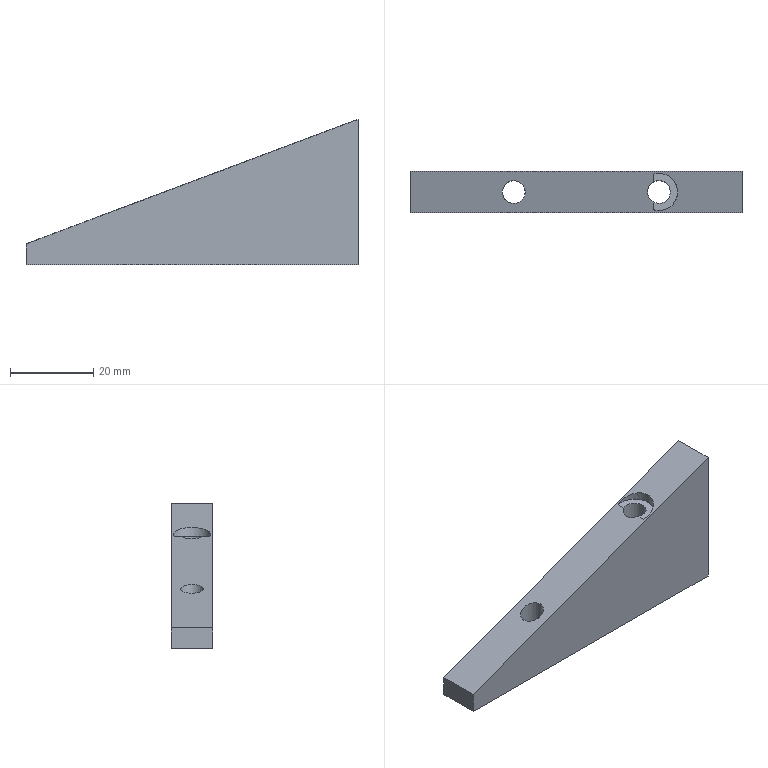Part | NX | 1 solid | 12 faces | box 80 x 10 x 35 mm | volume 14711 mm3 | plane 7 | cylinder 4 | cone 1 | commonest cylinder face diameters 5.5 x2 5 x1 9 x1
STEP:
#1=CARTESIAN_POINT('',(58.667,0.7021,27.));
#2=VERTEX_POINT('',#1);
#3=CARTESIAN_POINT('',(58.667,9.298,27.));
#4=VERTEX_POINT('',#3);
#5=CARTESIAN_POINT('',(60.,5.,27.));
#6=DIRECTION('',(0.,0.,1.));
#7=DIRECTION('',(1.,0.,0.));
#8=AXIS2_PLACEMENT_3D('',#5,#6,#7);
#9=CIRCLE('',#8,4.5);
#10=EDGE_CURVE('',#2,#4,#9,.T.);
#11=ORIENTED_EDGE('',*,*,#10,.F.);
#12=CARTESIAN_POINT('',(64.5,5.,29.188));
#13=VERTEX_POINT('',#12);
#14=CARTESIAN_POINT('',(58.667,0.7021,27.));
#15=CARTESIAN_POINT('',(61.832,-0.2799,28.187));
#16=CARTESIAN_POINT('',(64.5,1.686,29.188));
#17=CARTESIAN_POINT('',(64.5,5.,29.188));
#18=(BOUNDED_CURVE()B_SPLINE_CURVE(3,(#14,#15,#16,#17),.UNSPECIFIED.,.F.,.F.)B_SPLINE_CURVE_WITH_KNOTS((4,4),(0.,1.),.PIECEWISE_BEZIER_KNOTS.)CURVE()GEOMETRIC_REPRESENTATION_ITEM()RATIONAL_B_SPLINE_CURVE((1.,0.7288,0.7288,1.))REPRESENTATION_ITEM(''));
#19=EDGE_CURVE('',#2,#13,#18,.T.);
#20=ORIENTED_EDGE('',*,*,#19,.T.);
#21=CARTESIAN_POINT('',(64.5,5.,29.188));
#22=CARTESIAN_POINT('',(64.5,8.314,29.188));
#23=CARTESIAN_POINT('',(61.832,10.28,28.187));
#24=CARTESIAN_POINT('',(58.667,9.298,27.));
#25=(BOUNDED_CURVE()B_SPLINE_CURVE(3,(#21,#22,#23,#24),.UNSPECIFIED.,.F.,.F.)B_SPLINE_CURVE_WITH_KNOTS((4,4),(0.,1.),.PIECEWISE_BEZIER_KNOTS.)CURVE()GEOMETRIC_REPRESENTATION_ITEM()RATIONAL_B_SPLINE_CURVE((1.,0.7288,0.7288,1.))REPRESENTATION_ITEM(''));
#26=EDGE_CURVE('',#13,#4,#25,.T.);
#27=ORIENTED_EDGE('',*,*,#26,.T.);
#28=EDGE_LOOP('',(#11,#20,#27));
#29=FACE_BOUND('',#28,.T.);
#30=CARTESIAN_POINT('',(60.,5.,27.));
#31=DIRECTION('',(0.,0.,1.));
#32=DIRECTION('',(-1.,0.,0.));
#33=AXIS2_PLACEMENT_3D('',#30,#31,#32);
#34=CYLINDRICAL_SURFACE('',#33,4.5);
#35=ADVANCED_FACE('',(#29),#34,.F.);
#36=CARTESIAN_POINT('',(80.,5.,20.5));
#37=VERTEX_POINT('',#36);
#38=CARTESIAN_POINT('',(80.,5.,23.));
#39=DIRECTION('',(1.,0.,0.));
#40=DIRECTION('',(0.,0.,-1.));
#41=AXIS2_PLACEMENT_3D('',#38,#39,#40);
#42=CIRCLE('',#41,2.5);
#43=EDGE_CURVE('',#37,#37,#42,.T.);
#44=ORIENTED_EDGE('',*,*,#43,.T.);
#45=EDGE_LOOP('',(#44));
#46=FACE_BOUND('',#45,.T.);
#47=CARTESIAN_POINT('',(67.,5.,20.5));
#48=VERTEX_POINT('',#47);
#49=CARTESIAN_POINT('',(67.,5.,23.));
#50=DIRECTION('',(1.,0.,0.));
#51=DIRECTION('',(0.,0.,-1.));
#52=AXIS2_PLACEMENT_3D('',#49,#50,#51);
#53=CIRCLE('',#52,2.5);
#54=EDGE_CURVE('',#48,#48,#53,.T.);
#55=ORIENTED_EDGE('',*,*,#54,.F.);
#56=EDGE_LOOP('',(#55));
#57=FACE_BOUND('',#56,.T.);
#58=CARTESIAN_POINT('',(80.,5.,23.));
#59=DIRECTION('',(1.,0.,0.));
#60=DIRECTION('',(0.,0.,1.));
#61=AXIS2_PLACEMENT_3D('',#58,#59,#60);
#62=CYLINDRICAL_SURFACE('',#61,2.5);
#63=ADVANCED_FACE('',(#46,#57),#62,.F.);
#64=ORIENTED_EDGE('',*,*,#54,.T.);
#65=EDGE_LOOP('',(#64));
#66=FACE_BOUND('',#65,.T.);
#67=CARTESIAN_POINT('',(65.498,5.,23.));
#68=VERTEX_POINT('',#67);
#69=VERTEX_LOOP('',#68);
#70=FACE_BOUND('',#69,.T.);
#71=CARTESIAN_POINT('',(67.,5.,23.));
#72=DIRECTION('',(1.,0.,0.));
#73=DIRECTION('',(0.,0.,1.));
#74=AXIS2_PLACEMENT_3D('',#71,#72,#73);
#75=CONICAL_SURFACE('',#74,2.5,1.03);
#76=ADVANCED_FACE('',(#66,#70),#75,.F.);
#77=CARTESIAN_POINT('',(22.25,5.,0.));
#78=VERTEX_POINT('',#77);
#79=CARTESIAN_POINT('',(25.,5.,0.));
#80=DIRECTION('',(0.,0.,-1.));
#81=DIRECTION('',(-1.,0.,0.));
#82=AXIS2_PLACEMENT_3D('',#79,#80,#81);
#83=CIRCLE('',#82,2.75);
#84=EDGE_CURVE('',#78,#78,#83,.T.);
#85=ORIENTED_EDGE('',*,*,#84,.T.);
#86=EDGE_LOOP('',(#85));
#87=FACE_BOUND('',#86,.T.);
#88=CARTESIAN_POINT('',(22.25,5.,13.344));
#89=VERTEX_POINT('',#88);
#90=CARTESIAN_POINT('',(27.75,5.,15.406));
#91=VERTEX_POINT('',#90);
#92=CARTESIAN_POINT('',(22.25,5.,13.344));
#93=CARTESIAN_POINT('',(22.25,-0.5,13.344));
#94=CARTESIAN_POINT('',(27.75,-0.5,15.406));
#95=CARTESIAN_POINT('',(27.75,5.,15.406));
#96=(BOUNDED_CURVE()B_SPLINE_CURVE(3,(#92,#93,#94,#95),.UNSPECIFIED.,.F.,.F.)B_SPLINE_CURVE_WITH_KNOTS((4,4),(0.,1.),.PIECEWISE_BEZIER_KNOTS.)CURVE()GEOMETRIC_REPRESENTATION_ITEM()RATIONAL_B_SPLINE_CURVE((1.,0.3333,0.3333,1.))REPRESENTATION_ITEM(''));
#97=EDGE_CURVE('',#89,#91,#96,.T.);
#98=ORIENTED_EDGE('',*,*,#97,.T.);
#99=CARTESIAN_POINT('',(27.75,5.,15.406));
#100=CARTESIAN_POINT('',(27.75,10.5,15.406));
#101=CARTESIAN_POINT('',(22.25,10.5,13.344));
#102=CARTESIAN_POINT('',(22.25,5.,13.344));
#103=(BOUNDED_CURVE()B_SPLINE_CURVE(3,(#99,#100,#101,#102),.UNSPECIFIED.,.F.,.F.)B_SPLINE_CURVE_WITH_KNOTS((4,4),(0.,1.),.PIECEWISE_BEZIER_KNOTS.)CURVE()GEOMETRIC_REPRESENTATION_ITEM()RATIONAL_B_SPLINE_CURVE((1.,0.3333,0.3333,1.))REPRESENTATION_ITEM(''));
#104=EDGE_CURVE('',#91,#89,#103,.T.);
#105=ORIENTED_EDGE('',*,*,#104,.T.);
#106=EDGE_LOOP('',(#98,#105));
#107=FACE_BOUND('',#106,.T.);
#108=CARTESIAN_POINT('',(25.,5.,35.));
#109=DIRECTION('',(0.,0.,-1.));
#110=DIRECTION('',(1.,0.,0.));
#111=AXIS2_PLACEMENT_3D('',#108,#109,#110);
#112=CYLINDRICAL_SURFACE('',#111,2.75);
#113=ADVANCED_FACE('',(#87,#107),#112,.F.);
#114=CARTESIAN_POINT('',(57.25,5.,0.));
#115=VERTEX_POINT('',#114);
#116=CARTESIAN_POINT('',(60.,5.,0.));
#117=DIRECTION('',(0.,0.,-1.));
#118=DIRECTION('',(-1.,0.,0.));
#119=AXIS2_PLACEMENT_3D('',#116,#117,#118);
#120=CIRCLE('',#119,2.75);
#121=EDGE_CURVE('',#115,#115,#120,.T.);
#122=ORIENTED_EDGE('',*,*,#121,.T.);
#123=EDGE_LOOP('',(#122));
#124=FACE_BOUND('',#123,.T.);
#125=CARTESIAN_POINT('',(58.667,7.405,27.));
#126=VERTEX_POINT('',#125);
#127=CARTESIAN_POINT('',(58.667,2.595,27.));
#128=VERTEX_POINT('',#127);
#129=CARTESIAN_POINT('',(60.,5.,27.));
#130=DIRECTION('',(0.,0.,-1.));
#131=DIRECTION('',(1.,0.,0.));
#132=AXIS2_PLACEMENT_3D('',#129,#130,#131);
#133=CIRCLE('',#132,2.75);
#134=EDGE_CURVE('',#126,#128,#133,.T.);
#135=ORIENTED_EDGE('',*,*,#134,.F.);
#136=CARTESIAN_POINT('',(57.25,5.,26.469));
#137=VERTEX_POINT('',#136);
#138=CARTESIAN_POINT('',(58.667,7.405,27.));
#139=CARTESIAN_POINT('',(57.77,6.908,26.664));
#140=CARTESIAN_POINT('',(57.25,6.025,26.469));
#141=CARTESIAN_POINT('',(57.25,5.,26.469));
#142=(BOUNDED_CURVE()B_SPLINE_CURVE(3,(#138,#139,#140,#141),.UNSPECIFIED.,.F.,.F.)B_SPLINE_CURVE_WITH_KNOTS((4,4),(0.,1.),.PIECEWISE_BEZIER_KNOTS.)CURVE()GEOMETRIC_REPRESENTATION_ITEM()RATIONAL_B_SPLINE_CURVE((1.,0.9078,0.9078,1.))REPRESENTATION_ITEM(''));
#143=EDGE_CURVE('',#126,#137,#142,.T.);
#144=ORIENTED_EDGE('',*,*,#143,.T.);
#145=CARTESIAN_POINT('',(57.25,5.,26.469));
#146=CARTESIAN_POINT('',(57.25,3.975,26.469));
#147=CARTESIAN_POINT('',(57.77,3.092,26.664));
#148=CARTESIAN_POINT('',(58.667,2.595,27.));
#149=(BOUNDED_CURVE()B_SPLINE_CURVE(3,(#145,#146,#147,#148),.UNSPECIFIED.,.F.,.F.)B_SPLINE_CURVE_WITH_KNOTS((4,4),(0.,1.),.PIECEWISE_BEZIER_KNOTS.)CURVE()GEOMETRIC_REPRESENTATION_ITEM()RATIONAL_B_SPLINE_CURVE((1.,0.9078,0.9078,1.))REPRESENTATION_ITEM(''));
#150=EDGE_CURVE('',#137,#128,#149,.T.);
#151=ORIENTED_EDGE('',*,*,#150,.T.);
#152=EDGE_LOOP('',(#135,#144,#151));
#153=FACE_BOUND('',#152,.T.);
#154=CARTESIAN_POINT('',(60.,5.,35.));
#155=DIRECTION('',(0.,0.,-1.));
#156=DIRECTION('',(1.,0.,0.));
#157=AXIS2_PLACEMENT_3D('',#154,#155,#156);
#158=CYLINDRICAL_SURFACE('',#157,2.75);
#159=ADVANCED_FACE('',(#124,#153),#158,.F.);
#160=CARTESIAN_POINT('',(0.,0.,0.));
#161=VERTEX_POINT('',#160);
#162=CARTESIAN_POINT('',(0.,0.,5.));
#163=VERTEX_POINT('',#162);
#164=CARTESIAN_POINT('',(0.,0.,35.));
#165=DIRECTION('',(0.,0.,1.));
#166=VECTOR('',#165,1000.);
#167=LINE('',#164,#166);
#168=EDGE_CURVE('',#161,#163,#167,.T.);
#169=ORIENTED_EDGE('',*,*,#168,.T.);
#170=CARTESIAN_POINT('',(0.,10.,5.));
#171=VERTEX_POINT('',#170);
#172=CARTESIAN_POINT('',(0.,10.,5.));
#173=DIRECTION('',(0.,-1.,0.));
#174=VECTOR('',#173,1000.);
#175=LINE('',#172,#174);
#176=EDGE_CURVE('',#171,#163,#175,.T.);
#177=ORIENTED_EDGE('',*,*,#176,.F.);
#178=CARTESIAN_POINT('',(0.,10.,0.));
#179=VERTEX_POINT('',#178);
#180=CARTESIAN_POINT('',(0.,10.,5.));
#181=DIRECTION('',(0.,0.,1.));
#182=VECTOR('',#181,1000.);
#183=LINE('',#180,#182);
#184=EDGE_CURVE('',#179,#171,#183,.T.);
#185=ORIENTED_EDGE('',*,*,#184,.F.);
#186=CARTESIAN_POINT('',(0.,10.,0.));
#187=DIRECTION('',(0.,-1.,0.));
#188=VECTOR('',#187,1000.);
#189=LINE('',#186,#188);
#190=EDGE_CURVE('',#179,#161,#189,.T.);
#191=ORIENTED_EDGE('',*,*,#190,.T.);
#192=EDGE_LOOP('',(#169,#177,#185,#191));
#193=FACE_BOUND('',#192,.T.);
#194=CARTESIAN_POINT('',(0.,10.,35.));
#195=DIRECTION('',(1.,0.,0.));
#196=DIRECTION('',(0.,0.,1.));
#197=AXIS2_PLACEMENT_3D('',#194,#195,#196);
#198=PLANE('',#197);
#199=ADVANCED_FACE('',(#193),#198,.F.);
#200=ORIENTED_EDGE('',*,*,#43,.F.);
#201=EDGE_LOOP('',(#200));
#202=FACE_BOUND('',#201,.T.);
#203=CARTESIAN_POINT('',(80.,0.,35.));
#204=VERTEX_POINT('',#203);
#205=CARTESIAN_POINT('',(80.,0.,0.));
#206=VERTEX_POINT('',#205);
#207=CARTESIAN_POINT('',(80.,0.,0.));
#208=DIRECTION('',(0.,0.,-1.));
#209=VECTOR('',#208,1000.);
#210=LINE('',#207,#209);
#211=EDGE_CURVE('',#204,#206,#210,.T.);
#212=ORIENTED_EDGE('',*,*,#211,.T.);
#213=CARTESIAN_POINT('',(80.,10.,0.));
#214=VERTEX_POINT('',#213);
#215=CARTESIAN_POINT('',(80.,10.,0.));
#216=DIRECTION('',(0.,-1.,0.));
#217=VECTOR('',#216,1000.);
#218=LINE('',#215,#217);
#219=EDGE_CURVE('',#214,#206,#218,.T.);
#220=ORIENTED_EDGE('',*,*,#219,.F.);
#221=CARTESIAN_POINT('',(80.,10.,35.));
#222=VERTEX_POINT('',#221);
#223=CARTESIAN_POINT('',(80.,10.,0.));
#224=DIRECTION('',(0.,0.,-1.));
#225=VECTOR('',#224,1000.);
#226=LINE('',#223,#225);
#227=EDGE_CURVE('',#222,#214,#226,.T.);
#228=ORIENTED_EDGE('',*,*,#227,.F.);
#229=CARTESIAN_POINT('',(80.,10.,35.));
#230=DIRECTION('',(0.,-1.,0.));
#231=VECTOR('',#230,1000.);
#232=LINE('',#229,#231);
#233=EDGE_CURVE('',#222,#204,#232,.T.);
#234=ORIENTED_EDGE('',*,*,#233,.T.);
#235=EDGE_LOOP('',(#212,#220,#228,#234));
#236=FACE_BOUND('',#235,.T.);
#237=CARTESIAN_POINT('',(80.,10.,0.));
#238=DIRECTION('',(-1.,0.,0.));
#239=DIRECTION('',(0.,0.,-1.));
#240=AXIS2_PLACEMENT_3D('',#237,#238,#239);
#241=PLANE('',#240);
#242=ADVANCED_FACE('',(#202,#236),#241,.F.);
#243=ORIENTED_EDGE('',*,*,#84,.F.);
#244=EDGE_LOOP('',(#243));
#245=FACE_BOUND('',#244,.T.);
#246=ORIENTED_EDGE('',*,*,#121,.F.);
#247=EDGE_LOOP('',(#246));
#248=FACE_BOUND('',#247,.T.);
#249=CARTESIAN_POINT('',(0.,0.,0.));
#250=DIRECTION('',(-1.,0.,0.));
#251=VECTOR('',#250,1000.);
#252=LINE('',#249,#251);
#253=EDGE_CURVE('',#206,#161,#252,.T.);
#254=ORIENTED_EDGE('',*,*,#253,.T.);
#255=ORIENTED_EDGE('',*,*,#190,.F.);
#256=CARTESIAN_POINT('',(0.,10.,0.));
#257=DIRECTION('',(-1.,0.,0.));
#258=VECTOR('',#257,1000.);
#259=LINE('',#256,#258);
#260=EDGE_CURVE('',#214,#179,#259,.T.);
#261=ORIENTED_EDGE('',*,*,#260,.F.);
#262=ORIENTED_EDGE('',*,*,#219,.T.);
#263=EDGE_LOOP('',(#254,#255,#261,#262));
#264=FACE_BOUND('',#263,.T.);
#265=CARTESIAN_POINT('',(0.,10.,0.));
#266=DIRECTION('',(0.,0.,1.));
#267=DIRECTION('',(-1.,0.,0.));
#268=AXIS2_PLACEMENT_3D('',#265,#266,#267);
#269=PLANE('',#268);
#270=ADVANCED_FACE('',(#245,#248,#264),#269,.F.);
#271=ORIENTED_EDGE('',*,*,#184,.T.);
#272=CARTESIAN_POINT('',(0.,10.,5.));
#273=DIRECTION('',(0.9363,0.,0.3511));
#274=VECTOR('',#273,1000.);
#275=LINE('',#272,#274);
#276=EDGE_CURVE('',#171,#222,#275,.T.);
#277=ORIENTED_EDGE('',*,*,#276,.T.);
#278=ORIENTED_EDGE('',*,*,#227,.T.);
#279=ORIENTED_EDGE('',*,*,#260,.T.);
#280=EDGE_LOOP('',(#271,#277,#278,#279));
#281=FACE_BOUND('',#280,.T.);
#282=CARTESIAN_POINT('',(0.,10.,0.));
#283=DIRECTION('',(0.,-1.,0.));
#284=DIRECTION('',(0.,0.,1.));
#285=AXIS2_PLACEMENT_3D('',#282,#283,#284);
#286=PLANE('',#285);
#287=ADVANCED_FACE('',(#281),#286,.F.);
#288=CARTESIAN_POINT('',(0.,0.,5.));
#289=DIRECTION('',(0.9363,0.,0.3511));
#290=VECTOR('',#289,1000.);
#291=LINE('',#288,#290);
#292=EDGE_CURVE('',#163,#204,#291,.T.);
#293=ORIENTED_EDGE('',*,*,#292,.F.);
#294=ORIENTED_EDGE('',*,*,#168,.F.);
#295=ORIENTED_EDGE('',*,*,#253,.F.);
#296=ORIENTED_EDGE('',*,*,#211,.F.);
#297=EDGE_LOOP('',(#293,#294,#295,#296));
#298=FACE_BOUND('',#297,.T.);
#299=CARTESIAN_POINT('',(0.,0.,0.));
#300=DIRECTION('',(0.,-1.,0.));
#301=DIRECTION('',(0.,0.,1.));
#302=AXIS2_PLACEMENT_3D('',#299,#300,#301);
#303=PLANE('',#302);
#304=ADVANCED_FACE('',(#298),#303,.T.);
#305=CARTESIAN_POINT('',(58.667,5.,27.));
#306=DIRECTION('',(0.,1.,0.));
#307=VECTOR('',#306,1000.);
#308=LINE('',#305,#307);
#309=EDGE_CURVE('',#2,#128,#308,.T.);
#310=ORIENTED_EDGE('',*,*,#309,.F.);
#311=ORIENTED_EDGE('',*,*,#10,.T.);
#312=CARTESIAN_POINT('',(58.667,5.,27.));
#313=DIRECTION('',(0.,1.,0.));
#314=VECTOR('',#313,1000.);
#315=LINE('',#312,#314);
#316=EDGE_CURVE('',#126,#4,#315,.T.);
#317=ORIENTED_EDGE('',*,*,#316,.F.);
#318=ORIENTED_EDGE('',*,*,#134,.T.);
#319=EDGE_LOOP('',(#310,#311,#317,#318));
#320=FACE_BOUND('',#319,.T.);
#321=CARTESIAN_POINT('',(60.,5.,27.));
#322=DIRECTION('',(0.,0.,1.));
#323=DIRECTION('',(-1.,0.,0.));
#324=AXIS2_PLACEMENT_3D('',#321,#322,#323);
#325=PLANE('',#324);
#326=ADVANCED_FACE('',(#320),#325,.T.);
#327=ORIENTED_EDGE('',*,*,#316,.T.);
#328=ORIENTED_EDGE('',*,*,#26,.F.);
#329=ORIENTED_EDGE('',*,*,#19,.F.);
#330=ORIENTED_EDGE('',*,*,#309,.T.);
#331=ORIENTED_EDGE('',*,*,#150,.F.);
#332=ORIENTED_EDGE('',*,*,#143,.F.);
#333=EDGE_LOOP('',(#327,#328,#329,#330,#331,#332));
#334=FACE_BOUND('',#333,.T.);
#335=ORIENTED_EDGE('',*,*,#292,.T.);
#336=ORIENTED_EDGE('',*,*,#233,.F.);
#337=ORIENTED_EDGE('',*,*,#276,.F.);
#338=ORIENTED_EDGE('',*,*,#176,.T.);
#339=EDGE_LOOP('',(#335,#336,#337,#338));
#340=FACE_BOUND('',#339,.T.);
#341=ORIENTED_EDGE('',*,*,#97,.F.);
#342=ORIENTED_EDGE('',*,*,#104,.F.);
#343=EDGE_LOOP('',(#341,#342));
#344=FACE_BOUND('',#343,.T.);
#345=CARTESIAN_POINT('',(0.,10.,5.));
#346=DIRECTION('',(0.3511,0.,-0.9363));
#347=DIRECTION('',(0.9363,0.,0.3511));
#348=AXIS2_PLACEMENT_3D('',#345,#346,#347);
#349=PLANE('',#348);
#350=ADVANCED_FACE('',(#334,#340,#344),#349,.F.);
#351=CLOSED_SHELL('',(#35,#63,#76,#113,#159,#199,#242,#270,#287,#304,#326,#350));
#352=MANIFOLD_SOLID_BREP('',#351);
#353=(LENGTH_UNIT()NAMED_UNIT(*)SI_UNIT(.MILLI.,.METRE.));
#354=UNCERTAINTY_MEASURE_WITH_UNIT(LENGTH_MEASURE(0.00001),#353,'','');
#355=(NAMED_UNIT(*)PLANE_ANGLE_UNIT()SI_UNIT($,.RADIAN.));
#356=(NAMED_UNIT(*)SI_UNIT($,.STERADIAN.)SOLID_ANGLE_UNIT());
#357=(GEOMETRIC_REPRESENTATION_CONTEXT(3)GLOBAL_UNCERTAINTY_ASSIGNED_CONTEXT((#354))GLOBAL_UNIT_ASSIGNED_CONTEXT((#353,#355,#356))REPRESENTATION_CONTEXT('',''));
#358=ADVANCED_BREP_SHAPE_REPRESENTATION('',(#352),#357);